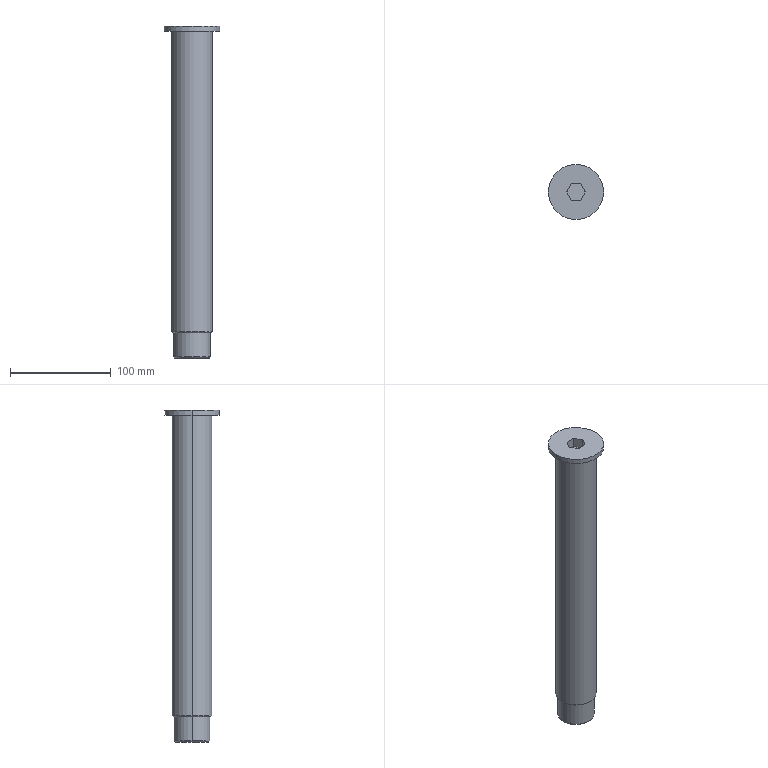Part | SolidWorks | features ICE 4, Chamfer 2, Fillet 2, Extrusion 1 | 1 solid | 32 faces | box 55 x 55 x 330 mm | volume 411254 mm3 | plane 14 | cylinder 11 | cone 5 | torus 2 | commonest cylinder face diameters 1 x4 36 x3 40 x2 55 x2
STEP:
#1=CARTESIAN_POINT('',(-20.5,0.,325.));
#2=VERTEX_POINT('',#1);
#3=CARTESIAN_POINT('',(20.5,0.,325.));
#4=VERTEX_POINT('',#3);
#5=CARTESIAN_POINT('',(0.,0.,325.));
#6=DIRECTION('',(0.,0.,1.));
#7=DIRECTION('',(1.,0.,0.));
#8=AXIS2_PLACEMENT_3D('',#5,#6,#7);
#9=CIRCLE('',#8,20.5);
#10=EDGE_CURVE('',#2,#4,#9,.T.);
#11=ORIENTED_EDGE('',*,*,#10,.F.);
#12=CARTESIAN_POINT('',(-20.,0.,324.5));
#13=VERTEX_POINT('',#12);
#14=CARTESIAN_POINT('',(-20.5,0.,324.5));
#15=DIRECTION('',(0.,1.,0.));
#16=DIRECTION('',(-1.,0.,0.));
#17=AXIS2_PLACEMENT_3D('',#14,#15,#16);
#18=CIRCLE('',#17,0.5);
#19=EDGE_CURVE('',#2,#13,#18,.T.);
#20=ORIENTED_EDGE('',*,*,#19,.T.);
#21=CARTESIAN_POINT('',(20.,0.,324.5));
#22=VERTEX_POINT('',#21);
#23=CARTESIAN_POINT('',(0.,0.,324.5));
#24=DIRECTION('',(0.,0.,-1.));
#25=DIRECTION('',(1.,0.,0.));
#26=AXIS2_PLACEMENT_3D('',#23,#24,#25);
#27=CIRCLE('',#26,20.);
#28=EDGE_CURVE('',#22,#13,#27,.T.);
#29=ORIENTED_EDGE('',*,*,#28,.F.);
#30=CARTESIAN_POINT('',(20.5,0.,324.5));
#31=DIRECTION('',(0.,-1.,0.));
#32=DIRECTION('',(0.,0.,-1.));
#33=AXIS2_PLACEMENT_3D('',#30,#31,#32);
#34=CIRCLE('',#33,0.5);
#35=EDGE_CURVE('',#4,#22,#34,.T.);
#36=ORIENTED_EDGE('',*,*,#35,.F.);
#37=EDGE_LOOP('',(#11,#20,#29,#36));
#38=FACE_OUTER_BOUND('',#37,.T.);
#39=CARTESIAN_POINT('',(0.,0.,324.5));
#40=DIRECTION('',(0.,0.,1.));
#41=DIRECTION('',(1.,0.,0.));
#42=AXIS2_PLACEMENT_3D('',#39,#40,#41);
#43=TOROIDAL_SURFACE('',#42,20.5,0.5);
#44=ADVANCED_FACE('',(#38),#43,.F.);
#45=CARTESIAN_POINT('',(-17.,0.,0.));
#46=VERTEX_POINT('',#45);
#47=CARTESIAN_POINT('',(-3.,16.733,0.));
#48=VERTEX_POINT('',#47);
#49=CARTESIAN_POINT('',(0.,0.,0.));
#50=DIRECTION('',(0.,0.,-1.));
#51=DIRECTION('',(1.,0.,0.));
#52=AXIS2_PLACEMENT_3D('',#49,#50,#51);
#53=CIRCLE('',#52,17.);
#54=EDGE_CURVE('',#46,#48,#53,.T.);
#55=ORIENTED_EDGE('',*,*,#54,.F.);
#56=CARTESIAN_POINT('',(-18.,0.,1.));
#57=VERTEX_POINT('',#56);
#58=CARTESIAN_POINT('',(-17.,0.,0.));
#59=DIRECTION('',(-0.7071,0.,0.7071));
#60=VECTOR('',#59,1000.);
#61=LINE('',#58,#60);
#62=EDGE_CURVE('',#46,#57,#61,.T.);
#63=ORIENTED_EDGE('',*,*,#62,.T.);
#64=CARTESIAN_POINT('',(-3.6,17.636,1.));
#65=VERTEX_POINT('',#64);
#66=CARTESIAN_POINT('',(0.,0.,1.));
#67=DIRECTION('',(0.,0.,1.));
#68=DIRECTION('',(1.,0.,0.));
#69=AXIS2_PLACEMENT_3D('',#66,#67,#68);
#70=CIRCLE('',#69,18.);
#71=EDGE_CURVE('',#65,#57,#70,.T.);
#72=ORIENTED_EDGE('',*,*,#71,.F.);
#73=CARTESIAN_POINT('',(-3.,17.146,0.4069));
#74=VERTEX_POINT('',#73);
#75=CARTESIAN_POINT('',(-3.6,17.636,1.));
#76=CARTESIAN_POINT('',(-3.509,17.655,1.));
#77=CARTESIAN_POINT('',(-3.418,17.647,0.9743));
#78=CARTESIAN_POINT('',(-3.262,17.594,0.8932));
#79=CARTESIAN_POINT('',(-3.198,17.551,0.8399));
#80=CARTESIAN_POINT('',(-3.098,17.452,0.7251));
#81=CARTESIAN_POINT('',(-3.061,17.395,0.6623));
#82=CARTESIAN_POINT('',(-3.013,17.275,0.5357));
#83=CARTESIAN_POINT('',(-3.,17.212,0.4712));
#84=CARTESIAN_POINT('',(-3.,17.146,0.4069));
#85=B_SPLINE_CURVE_WITH_KNOTS('',3,(#75,#76,#77,#78,#79,#80,#81,#82,#83,#84),.UNSPECIFIED.,.F.,.F.,(4,2,2,2,4),(0.,0.0002726,0.0005452,0.0008178,0.00109),.UNSPECIFIED.);
#86=EDGE_CURVE('',#65,#74,#85,.T.);
#87=ORIENTED_EDGE('',*,*,#86,.T.);
#88=CARTESIAN_POINT('',(-3.,16.733,0.));
#89=CARTESIAN_POINT('',(-3.,16.871,0.1356));
#90=CARTESIAN_POINT('',(-3.,17.009,0.2712));
#91=CARTESIAN_POINT('',(-3.,17.146,0.4069));
#92=B_SPLINE_CURVE_WITH_KNOTS('',3,(#88,#89,#90,#91),.UNSPECIFIED.,.F.,.F.,(4,4),(0.007295,0.007875),.UNSPECIFIED.);
#93=EDGE_CURVE('',#48,#74,#92,.T.);
#94=ORIENTED_EDGE('',*,*,#93,.F.);
#95=EDGE_LOOP('',(#55,#63,#72,#87,#94));
#96=FACE_OUTER_BOUND('',#95,.T.);
#97=CARTESIAN_POINT('',(0.,0.,0.));
#98=DIRECTION('',(0.,0.,1.));
#99=DIRECTION('',(1.,0.,0.));
#100=AXIS2_PLACEMENT_3D('',#97,#98,#99);
#101=CONICAL_SURFACE('',#100,17.,0.7854);
#102=ADVANCED_FACE('',(#96),#101,.T.);
#103=ORIENTED_EDGE('',*,*,#62,.F.);
#104=CARTESIAN_POINT('',(17.,0.,0.));
#105=VERTEX_POINT('',#104);
#106=CARTESIAN_POINT('',(0.,0.,0.));
#107=DIRECTION('',(0.,0.,-1.));
#108=DIRECTION('',(1.,0.,0.));
#109=AXIS2_PLACEMENT_3D('',#106,#107,#108);
#110=CIRCLE('',#109,17.);
#111=EDGE_CURVE('',#105,#46,#110,.T.);
#112=ORIENTED_EDGE('',*,*,#111,.F.);
#113=CARTESIAN_POINT('',(18.,0.,1.));
#114=VERTEX_POINT('',#113);
#115=CARTESIAN_POINT('',(17.,0.,0.));
#116=DIRECTION('',(0.7071,0.,0.7071));
#117=VECTOR('',#116,1000.);
#118=LINE('',#115,#117);
#119=EDGE_CURVE('',#105,#114,#118,.T.);
#120=ORIENTED_EDGE('',*,*,#119,.T.);
#121=CARTESIAN_POINT('',(0.,0.,1.));
#122=DIRECTION('',(0.,0.,1.));
#123=DIRECTION('',(1.,0.,0.));
#124=AXIS2_PLACEMENT_3D('',#121,#122,#123);
#125=CIRCLE('',#124,18.);
#126=EDGE_CURVE('',#57,#114,#125,.T.);
#127=ORIENTED_EDGE('',*,*,#126,.F.);
#128=EDGE_LOOP('',(#103,#112,#120,#127));
#129=FACE_OUTER_BOUND('',#128,.T.);
#130=CARTESIAN_POINT('',(0.,0.,0.));
#131=DIRECTION('',(0.,0.,1.));
#132=DIRECTION('',(1.,0.,0.));
#133=AXIS2_PLACEMENT_3D('',#130,#131,#132);
#134=CONICAL_SURFACE('',#133,17.,0.7854);
#135=ADVANCED_FACE('',(#129),#134,.T.);
#136=CARTESIAN_POINT('',(-19.,0.,25.));
#137=VERTEX_POINT('',#136);
#138=CARTESIAN_POINT('',(19.,0.,25.));
#139=VERTEX_POINT('',#138);
#140=CARTESIAN_POINT('',(0.,0.,25.));
#141=DIRECTION('',(0.,0.,-1.));
#142=DIRECTION('',(-1.,0.,0.));
#143=AXIS2_PLACEMENT_3D('',#140,#141,#142);
#144=CIRCLE('',#143,19.);
#145=EDGE_CURVE('',#137,#139,#144,.T.);
#146=ORIENTED_EDGE('',*,*,#145,.F.);
#147=CARTESIAN_POINT('',(-20.,0.,26.));
#148=VERTEX_POINT('',#147);
#149=CARTESIAN_POINT('',(-19.,0.,25.));
#150=DIRECTION('',(-0.7071,0.,0.7071));
#151=VECTOR('',#150,1000.);
#152=LINE('',#149,#151);
#153=EDGE_CURVE('',#137,#148,#152,.T.);
#154=ORIENTED_EDGE('',*,*,#153,.T.);
#155=CARTESIAN_POINT('',(20.,0.,26.));
#156=VERTEX_POINT('',#155);
#157=CARTESIAN_POINT('',(0.,0.,26.));
#158=DIRECTION('',(0.,0.,1.));
#159=DIRECTION('',(-1.,0.,0.));
#160=AXIS2_PLACEMENT_3D('',#157,#158,#159);
#161=CIRCLE('',#160,20.);
#162=EDGE_CURVE('',#156,#148,#161,.T.);
#163=ORIENTED_EDGE('',*,*,#162,.F.);
#164=CARTESIAN_POINT('',(19.,0.,25.));
#165=DIRECTION('',(0.7071,0.,0.7071));
#166=VECTOR('',#165,1000.);
#167=LINE('',#164,#166);
#168=EDGE_CURVE('',#139,#156,#167,.T.);
#169=ORIENTED_EDGE('',*,*,#168,.F.);
#170=EDGE_LOOP('',(#146,#154,#163,#169));
#171=FACE_OUTER_BOUND('',#170,.T.);
#172=CARTESIAN_POINT('',(0.,0.,25.));
#173=DIRECTION('',(0.,0.,1.));
#174=DIRECTION('',(1.,0.,0.));
#175=AXIS2_PLACEMENT_3D('',#172,#173,#174);
#176=CONICAL_SURFACE('',#175,19.,0.7854);
#177=ADVANCED_FACE('',(#171),#176,.T.);
#178=CARTESIAN_POINT('',(3.6,17.636,25.));
#179=VERTEX_POINT('',#178);
#180=CARTESIAN_POINT('',(18.,0.,25.));
#181=VERTEX_POINT('',#180);
#182=CARTESIAN_POINT('',(0.,0.,25.));
#183=DIRECTION('',(0.,0.,-1.));
#184=DIRECTION('',(-1.,0.,0.));
#185=AXIS2_PLACEMENT_3D('',#182,#183,#184);
#186=CIRCLE('',#185,18.);
#187=EDGE_CURVE('',#179,#181,#186,.T.);
#188=ORIENTED_EDGE('',*,*,#187,.T.);
#189=CARTESIAN_POINT('',(18.,0.,25.));
#190=DIRECTION('',(0.,0.,-1.));
#191=VECTOR('',#190,1000.);
#192=LINE('',#189,#191);
#193=EDGE_CURVE('',#181,#114,#192,.T.);
#194=ORIENTED_EDGE('',*,*,#193,.T.);
#195=CARTESIAN_POINT('',(3.6,17.636,1.));
#196=VERTEX_POINT('',#195);
#197=CARTESIAN_POINT('',(0.,0.,1.));
#198=DIRECTION('',(0.,0.,1.));
#199=DIRECTION('',(1.,0.,0.));
#200=AXIS2_PLACEMENT_3D('',#197,#198,#199);
#201=CIRCLE('',#200,18.);
#202=EDGE_CURVE('',#114,#196,#201,.T.);
#203=ORIENTED_EDGE('',*,*,#202,.T.);
#204=CARTESIAN_POINT('',(3.6,17.636,25.));
#205=DIRECTION('',(0.,0.,1.));
#206=VECTOR('',#205,1000.);
#207=LINE('',#204,#206);
#208=EDGE_CURVE('',#196,#179,#207,.T.);
#209=ORIENTED_EDGE('',*,*,#208,.T.);
#210=EDGE_LOOP('',(#188,#194,#203,#209));
#211=FACE_OUTER_BOUND('',#210,.T.);
#212=CARTESIAN_POINT('',(0.,0.,25.));
#213=DIRECTION('',(0.,0.,-1.));
#214=DIRECTION('',(-1.,0.,0.));
#215=AXIS2_PLACEMENT_3D('',#212,#213,#214);
#216=CYLINDRICAL_SURFACE('',#215,18.);
#217=ADVANCED_FACE('',(#211),#216,.T.);
#218=ORIENTED_EDGE('',*,*,#193,.F.);
#219=CARTESIAN_POINT('',(-18.,0.,25.));
#220=VERTEX_POINT('',#219);
#221=CARTESIAN_POINT('',(0.,0.,25.));
#222=DIRECTION('',(0.,0.,-1.));
#223=DIRECTION('',(-1.,0.,0.));
#224=AXIS2_PLACEMENT_3D('',#221,#222,#223);
#225=CIRCLE('',#224,18.);
#226=EDGE_CURVE('',#181,#220,#225,.T.);
#227=ORIENTED_EDGE('',*,*,#226,.T.);
#228=CARTESIAN_POINT('',(-18.,0.,25.));
#229=DIRECTION('',(0.,0.,-1.));
#230=VECTOR('',#229,1000.);
#231=LINE('',#228,#230);
#232=EDGE_CURVE('',#220,#57,#231,.T.);
#233=ORIENTED_EDGE('',*,*,#232,.T.);
#234=ORIENTED_EDGE('',*,*,#126,.T.);
#235=EDGE_LOOP('',(#218,#227,#233,#234));
#236=FACE_OUTER_BOUND('',#235,.T.);
#237=CARTESIAN_POINT('',(0.,0.,25.));
#238=DIRECTION('',(0.,0.,-1.));
#239=DIRECTION('',(-1.,0.,0.));
#240=AXIS2_PLACEMENT_3D('',#237,#238,#239);
#241=CYLINDRICAL_SURFACE('',#240,18.);
#242=ADVANCED_FACE('',(#236),#241,.T.);
#243=CARTESIAN_POINT('',(27.5,0.,330.));
#244=VERTEX_POINT('',#243);
#245=CARTESIAN_POINT('',(-27.5,0.,330.));
#246=VERTEX_POINT('',#245);
#247=CARTESIAN_POINT('',(0.,0.,330.));
#248=DIRECTION('',(0.,0.,1.));
#249=DIRECTION('',(1.,0.,0.));
#250=AXIS2_PLACEMENT_3D('',#247,#248,#249);
#251=CIRCLE('',#250,27.5);
#252=EDGE_CURVE('',#244,#246,#251,.T.);
#253=ORIENTED_EDGE('',*,*,#252,.F.);
#254=CARTESIAN_POINT('',(27.5,0.,325.));
#255=VERTEX_POINT('',#254);
#256=CARTESIAN_POINT('',(27.5,0.,330.));
#257=DIRECTION('',(0.,0.,-1.));
#258=VECTOR('',#257,1000.);
#259=LINE('',#256,#258);
#260=EDGE_CURVE('',#244,#255,#259,.T.);
#261=ORIENTED_EDGE('',*,*,#260,.T.);
#262=CARTESIAN_POINT('',(-27.5,0.,325.));
#263=VERTEX_POINT('',#262);
#264=CARTESIAN_POINT('',(0.,0.,325.));
#265=DIRECTION('',(0.,0.,1.));
#266=DIRECTION('',(1.,0.,0.));
#267=AXIS2_PLACEMENT_3D('',#264,#265,#266);
#268=CIRCLE('',#267,27.5);
#269=EDGE_CURVE('',#255,#263,#268,.T.);
#270=ORIENTED_EDGE('',*,*,#269,.T.);
#271=CARTESIAN_POINT('',(-27.5,0.,330.));
#272=DIRECTION('',(0.,0.,-1.));
#273=VECTOR('',#272,1000.);
#274=LINE('',#271,#273);
#275=EDGE_CURVE('',#246,#263,#274,.T.);
#276=ORIENTED_EDGE('',*,*,#275,.F.);
#277=EDGE_LOOP('',(#253,#261,#270,#276));
#278=FACE_OUTER_BOUND('',#277,.T.);
#279=CARTESIAN_POINT('',(0.,0.,330.));
#280=DIRECTION('',(0.,0.,-1.));
#281=DIRECTION('',(-1.,0.,0.));
#282=AXIS2_PLACEMENT_3D('',#279,#280,#281);
#283=CYLINDRICAL_SURFACE('',#282,27.5);
#284=ADVANCED_FACE('',(#278),#283,.T.);
#285=CARTESIAN_POINT('',(0.,0.,324.5));
#286=DIRECTION('',(0.,0.,-1.));
#287=DIRECTION('',(1.,0.,0.));
#288=AXIS2_PLACEMENT_3D('',#285,#286,#287);
#289=CIRCLE('',#288,20.);
#290=EDGE_CURVE('',#13,#22,#289,.T.);
#291=ORIENTED_EDGE('',*,*,#290,.T.);
#292=CARTESIAN_POINT('',(20.,0.,325.));
#293=DIRECTION('',(0.,0.,-1.));
#294=VECTOR('',#293,1000.);
#295=LINE('',#292,#294);
#296=EDGE_CURVE('',#22,#156,#295,.T.);
#297=ORIENTED_EDGE('',*,*,#296,.T.);
#298=ORIENTED_EDGE('',*,*,#162,.T.);
#299=CARTESIAN_POINT('',(-20.,0.,325.));
#300=DIRECTION('',(0.,0.,-1.));
#301=VECTOR('',#300,1000.);
#302=LINE('',#299,#301);
#303=EDGE_CURVE('',#13,#148,#302,.T.);
#304=ORIENTED_EDGE('',*,*,#303,.F.);
#305=EDGE_LOOP('',(#291,#297,#298,#304));
#306=FACE_OUTER_BOUND('',#305,.T.);
#307=CARTESIAN_POINT('',(0.,0.,325.));
#308=DIRECTION('',(0.,0.,-1.));
#309=DIRECTION('',(-1.,0.,0.));
#310=AXIS2_PLACEMENT_3D('',#307,#308,#309);
#311=CYLINDRICAL_SURFACE('',#310,20.);
#312=ADVANCED_FACE('',(#306),#311,.T.);
#313=ORIENTED_EDGE('',*,*,#296,.F.);
#314=ORIENTED_EDGE('',*,*,#28,.T.);
#315=ORIENTED_EDGE('',*,*,#303,.T.);
#316=CARTESIAN_POINT('',(0.,0.,26.));
#317=DIRECTION('',(0.,0.,1.));
#318=DIRECTION('',(-1.,0.,0.));
#319=AXIS2_PLACEMENT_3D('',#316,#317,#318);
#320=CIRCLE('',#319,20.);
#321=EDGE_CURVE('',#148,#156,#320,.T.);
#322=ORIENTED_EDGE('',*,*,#321,.T.);
#323=EDGE_LOOP('',(#313,#314,#315,#322));
#324=FACE_OUTER_BOUND('',#323,.T.);
#325=CARTESIAN_POINT('',(0.,0.,325.));
#326=DIRECTION('',(0.,0.,-1.));
#327=DIRECTION('',(-1.,0.,0.));
#328=AXIS2_PLACEMENT_3D('',#325,#326,#327);
#329=CYLINDRICAL_SURFACE('',#328,20.);
#330=ADVANCED_FACE('',(#324),#329,.T.);
#331=ORIENTED_EDGE('',*,*,#260,.F.);
#332=CARTESIAN_POINT('',(0.,0.,330.));
#333=DIRECTION('',(0.,0.,1.));
#334=DIRECTION('',(1.,0.,0.));
#335=AXIS2_PLACEMENT_3D('',#332,#333,#334);
#336=CIRCLE('',#335,27.5);
#337=EDGE_CURVE('',#246,#244,#336,.T.);
#338=ORIENTED_EDGE('',*,*,#337,.F.);
#339=ORIENTED_EDGE('',*,*,#275,.T.);
#340=CARTESIAN_POINT('',(0.,0.,325.));
#341=DIRECTION('',(0.,0.,1.));
#342=DIRECTION('',(1.,0.,0.));
#343=AXIS2_PLACEMENT_3D('',#340,#341,#342);
#344=CIRCLE('',#343,27.5);
#345=EDGE_CURVE('',#263,#255,#344,.T.);
#346=ORIENTED_EDGE('',*,*,#345,.T.);
#347=EDGE_LOOP('',(#331,#338,#339,#346));
#348=FACE_OUTER_BOUND('',#347,.T.);
#349=CARTESIAN_POINT('',(0.,0.,330.));
#350=DIRECTION('',(0.,0.,-1.));
#351=DIRECTION('',(-1.,0.,0.));
#352=AXIS2_PLACEMENT_3D('',#349,#350,#351);
#353=CYLINDRICAL_SURFACE('',#352,27.5);
#354=ADVANCED_FACE('',(#348),#353,.T.);
#355=CARTESIAN_POINT('',(4.619,-8.,330.));
#356=VERTEX_POINT('',#355);
#357=CARTESIAN_POINT('',(9.238,0.,330.));
#358=VERTEX_POINT('',#357);
#359=CARTESIAN_POINT('',(4.619,-8.,330.));
#360=DIRECTION('',(0.5,0.866,0.));
#361=VECTOR('',#360,1000.);
#362=LINE('',#359,#361);
#363=EDGE_CURVE('',#356,#358,#362,.T.);
#364=ORIENTED_EDGE('',*,*,#363,.F.);
#365=CARTESIAN_POINT('',(-4.619,-8.,330.));
#366=VERTEX_POINT('',#365);
#367=CARTESIAN_POINT('',(-4.619,-8.,330.));
#368=DIRECTION('',(1.,0.,0.));
#369=VECTOR('',#368,1000.);
#370=LINE('',#367,#369);
#371=EDGE_CURVE('',#366,#356,#370,.T.);
#372=ORIENTED_EDGE('',*,*,#371,.F.);
#373=CARTESIAN_POINT('',(-9.238,0.,330.));
#374=VERTEX_POINT('',#373);
#375=CARTESIAN_POINT('',(-9.238,0.,330.));
#376=DIRECTION('',(0.5,-0.866,0.));
#377=VECTOR('',#376,1000.);
#378=LINE('',#375,#377);
#379=EDGE_CURVE('',#374,#366,#378,.T.);
#380=ORIENTED_EDGE('',*,*,#379,.F.);
#381=CARTESIAN_POINT('',(-4.619,8.,330.));
#382=VERTEX_POINT('',#381);
#383=CARTESIAN_POINT('',(-4.619,8.,330.));
#384=DIRECTION('',(-0.5,-0.866,0.));
#385=VECTOR('',#384,1000.);
#386=LINE('',#383,#385);
#387=EDGE_CURVE('',#382,#374,#386,.T.);
#388=ORIENTED_EDGE('',*,*,#387,.F.);
#389=CARTESIAN_POINT('',(4.619,8.,330.));
#390=VERTEX_POINT('',#389);
#391=CARTESIAN_POINT('',(4.619,8.,330.));
#392=DIRECTION('',(-1.,0.,0.));
#393=VECTOR('',#392,1000.);
#394=LINE('',#391,#393);
#395=EDGE_CURVE('',#390,#382,#394,.T.);
#396=ORIENTED_EDGE('',*,*,#395,.F.);
#397=CARTESIAN_POINT('',(9.238,0.,330.));
#398=DIRECTION('',(-0.5,0.866,0.));
#399=VECTOR('',#398,1000.);
#400=LINE('',#397,#399);
#401=EDGE_CURVE('',#358,#390,#400,.T.);
#402=ORIENTED_EDGE('',*,*,#401,.F.);
#403=EDGE_LOOP('',(#364,#372,#380,#388,#396,#402));
#404=FACE_BOUND('',#403,.T.);
#405=ORIENTED_EDGE('',*,*,#337,.T.);
#406=ORIENTED_EDGE('',*,*,#252,.T.);
#407=EDGE_LOOP('',(#405,#406));
#408=FACE_OUTER_BOUND('',#407,.T.);
#409=CARTESIAN_POINT('',(0.,0.,330.));
#410=DIRECTION('',(0.,0.,1.));
#411=DIRECTION('',(1.,0.,0.));
#412=AXIS2_PLACEMENT_3D('',#409,#410,#411);
#413=PLANE('',#412);
#414=ADVANCED_FACE('',(#404,#408),#413,.T.);
#415=CARTESIAN_POINT('',(0.,0.,325.));
#416=DIRECTION('',(0.,0.,1.));
#417=DIRECTION('',(1.,0.,0.));
#418=AXIS2_PLACEMENT_3D('',#415,#416,#417);
#419=CIRCLE('',#418,20.5);
#420=EDGE_CURVE('',#4,#2,#419,.T.);
#421=ORIENTED_EDGE('',*,*,#420,.T.);
#422=ORIENTED_EDGE('',*,*,#10,.T.);
#423=EDGE_LOOP('',(#421,#422));
#424=FACE_BOUND('',#423,.T.);
#425=ORIENTED_EDGE('',*,*,#345,.F.);
#426=ORIENTED_EDGE('',*,*,#269,.F.);
#427=EDGE_LOOP('',(#425,#426));
#428=FACE_OUTER_BOUND('',#427,.T.);
#429=CARTESIAN_POINT('',(0.,0.,325.));
#430=DIRECTION('',(0.,0.,1.));
#431=DIRECTION('',(1.,0.,0.));
#432=AXIS2_PLACEMENT_3D('',#429,#430,#431);
#433=PLANE('',#432);
#434=ADVANCED_FACE('',(#424,#428),#433,.F.);
#435=ORIENTED_EDGE('',*,*,#363,.T.);
#436=CARTESIAN_POINT('',(9.238,0.,320.));
#437=VERTEX_POINT('',#436);
#438=CARTESIAN_POINT('',(9.238,0.,320.));
#439=DIRECTION('',(0.,0.,1.));
#440=VECTOR('',#439,1000.);
#441=LINE('',#438,#440);
#442=EDGE_CURVE('',#437,#358,#441,.T.);
#443=ORIENTED_EDGE('',*,*,#442,.F.);
#444=CARTESIAN_POINT('',(4.619,-8.,320.));
#445=VERTEX_POINT('',#444);
#446=CARTESIAN_POINT('',(4.619,-8.,320.));
#447=DIRECTION('',(0.5,0.866,0.));
#448=VECTOR('',#447,1000.);
#449=LINE('',#446,#448);
#450=EDGE_CURVE('',#445,#437,#449,.T.);
#451=ORIENTED_EDGE('',*,*,#450,.F.);
#452=CARTESIAN_POINT('',(4.619,-8.,320.));
#453=DIRECTION('',(0.,0.,1.));
#454=VECTOR('',#453,1000.);
#455=LINE('',#452,#454);
#456=EDGE_CURVE('',#445,#356,#455,.T.);
#457=ORIENTED_EDGE('',*,*,#456,.T.);
#458=EDGE_LOOP('',(#435,#443,#451,#457));
#459=FACE_OUTER_BOUND('',#458,.T.);
#460=CARTESIAN_POINT('',(4.619,-8.,320.));
#461=DIRECTION('',(0.866,-0.5,0.));
#462=DIRECTION('',(0.5,0.866,0.));
#463=AXIS2_PLACEMENT_3D('',#460,#461,#462);
#464=PLANE('',#463);
#465=ADVANCED_FACE('',(#459),#464,.F.);
#466=ORIENTED_EDGE('',*,*,#371,.T.);
#467=ORIENTED_EDGE('',*,*,#456,.F.);
#468=CARTESIAN_POINT('',(-4.619,-8.,320.));
#469=VERTEX_POINT('',#468);
#470=CARTESIAN_POINT('',(-4.619,-8.,320.));
#471=DIRECTION('',(1.,0.,0.));
#472=VECTOR('',#471,1000.);
#473=LINE('',#470,#472);
#474=EDGE_CURVE('',#469,#445,#473,.T.);
#475=ORIENTED_EDGE('',*,*,#474,.F.);
#476=CARTESIAN_POINT('',(-4.619,-8.,320.));
#477=DIRECTION('',(0.,0.,1.));
#478=VECTOR('',#477,1000.);
#479=LINE('',#476,#478);
#480=EDGE_CURVE('',#469,#366,#479,.T.);
#481=ORIENTED_EDGE('',*,*,#480,.T.);
#482=EDGE_LOOP('',(#466,#467,#475,#481));
#483=FACE_OUTER_BOUND('',#482,.T.);
#484=CARTESIAN_POINT('',(-4.619,-8.,320.));
#485=DIRECTION('',(0.,-1.,0.));
#486=DIRECTION('',(1.,0.,0.));
#487=AXIS2_PLACEMENT_3D('',#484,#485,#486);
#488=PLANE('',#487);
#489=ADVANCED_FACE('',(#483),#488,.F.);
#490=ORIENTED_EDGE('',*,*,#379,.T.);
#491=ORIENTED_EDGE('',*,*,#480,.F.);
#492=CARTESIAN_POINT('',(-9.238,0.,320.));
#493=VERTEX_POINT('',#492);
#494=CARTESIAN_POINT('',(-9.238,0.,320.));
#495=DIRECTION('',(0.5,-0.866,0.));
#496=VECTOR('',#495,1000.);
#497=LINE('',#494,#496);
#498=EDGE_CURVE('',#493,#469,#497,.T.);
#499=ORIENTED_EDGE('',*,*,#498,.F.);
#500=CARTESIAN_POINT('',(-9.238,0.,320.));
#501=DIRECTION('',(0.,0.,1.));
#502=VECTOR('',#501,1000.);
#503=LINE('',#500,#502);
#504=EDGE_CURVE('',#493,#374,#503,.T.);
#505=ORIENTED_EDGE('',*,*,#504,.T.);
#506=EDGE_LOOP('',(#490,#491,#499,#505));
#507=FACE_OUTER_BOUND('',#506,.T.);
#508=CARTESIAN_POINT('',(-9.238,0.,320.));
#509=DIRECTION('',(-0.866,-0.5,0.));
#510=DIRECTION('',(0.5,-0.866,0.));
#511=AXIS2_PLACEMENT_3D('',#508,#509,#510);
#512=PLANE('',#511);
#513=ADVANCED_FACE('',(#507),#512,.F.);
#514=ORIENTED_EDGE('',*,*,#387,.T.);
#515=ORIENTED_EDGE('',*,*,#504,.F.);
#516=CARTESIAN_POINT('',(-4.619,8.,320.));
#517=VERTEX_POINT('',#516);
#518=CARTESIAN_POINT('',(-4.619,8.,320.));
#519=DIRECTION('',(-0.5,-0.866,0.));
#520=VECTOR('',#519,1000.);
#521=LINE('',#518,#520);
#522=EDGE_CURVE('',#517,#493,#521,.T.);
#523=ORIENTED_EDGE('',*,*,#522,.F.);
#524=CARTESIAN_POINT('',(-4.619,8.,320.));
#525=DIRECTION('',(0.,0.,1.));
#526=VECTOR('',#525,1000.);
#527=LINE('',#524,#526);
#528=EDGE_CURVE('',#517,#382,#527,.T.);
#529=ORIENTED_EDGE('',*,*,#528,.T.);
#530=EDGE_LOOP('',(#514,#515,#523,#529));
#531=FACE_OUTER_BOUND('',#530,.T.);
#532=CARTESIAN_POINT('',(-4.619,8.,320.));
#533=DIRECTION('',(-0.866,0.5,0.));
#534=DIRECTION('',(-0.5,-0.866,0.));
#535=AXIS2_PLACEMENT_3D('',#532,#533,#534);
#536=PLANE('',#535);
#537=ADVANCED_FACE('',(#531),#536,.F.);
#538=ORIENTED_EDGE('',*,*,#395,.T.);
#539=ORIENTED_EDGE('',*,*,#528,.F.);
#540=CARTESIAN_POINT('',(4.619,8.,320.));
#541=VERTEX_POINT('',#540);
#542=CARTESIAN_POINT('',(4.619,8.,320.));
#543=DIRECTION('',(-1.,0.,0.));
#544=VECTOR('',#543,1000.);
#545=LINE('',#542,#544);
#546=EDGE_CURVE('',#541,#517,#545,.T.);
#547=ORIENTED_EDGE('',*,*,#546,.F.);
#548=CARTESIAN_POINT('',(4.619,8.,320.));
#549=DIRECTION('',(0.,0.,1.));
#550=VECTOR('',#549,1000.);
#551=LINE('',#548,#550);
#552=EDGE_CURVE('',#541,#390,#551,.T.);
#553=ORIENTED_EDGE('',*,*,#552,.T.);
#554=EDGE_LOOP('',(#538,#539,#547,#553));
#555=FACE_OUTER_BOUND('',#554,.T.);
#556=CARTESIAN_POINT('',(4.619,8.,320.));
#557=DIRECTION('',(0.,1.,0.));
#558=DIRECTION('',(0.,0.,1.));
#559=AXIS2_PLACEMENT_3D('',#556,#557,#558);
#560=PLANE('',#559);
#561=ADVANCED_FACE('',(#555),#560,.F.);
#562=ORIENTED_EDGE('',*,*,#401,.T.);
#563=ORIENTED_EDGE('',*,*,#552,.F.);
#564=CARTESIAN_POINT('',(9.238,0.,320.));
#565=DIRECTION('',(-0.5,0.866,0.));
#566=VECTOR('',#565,1000.);
#567=LINE('',#564,#566);
#568=EDGE_CURVE('',#437,#541,#567,.T.);
#569=ORIENTED_EDGE('',*,*,#568,.F.);
#570=ORIENTED_EDGE('',*,*,#442,.T.);
#571=EDGE_LOOP('',(#562,#563,#569,#570));
#572=FACE_OUTER_BOUND('',#571,.T.);
#573=CARTESIAN_POINT('',(9.238,0.,320.));
#574=DIRECTION('',(0.866,0.5,0.));
#575=DIRECTION('',(-0.5,0.866,0.));
#576=AXIS2_PLACEMENT_3D('',#573,#574,#575);
#577=PLANE('',#576);
#578=ADVANCED_FACE('',(#572),#577,.F.);
#579=ORIENTED_EDGE('',*,*,#450,.T.);
#580=ORIENTED_EDGE('',*,*,#568,.T.);
#581=ORIENTED_EDGE('',*,*,#546,.T.);
#582=ORIENTED_EDGE('',*,*,#522,.T.);
#583=ORIENTED_EDGE('',*,*,#498,.T.);
#584=ORIENTED_EDGE('',*,*,#474,.T.);
#585=EDGE_LOOP('',(#579,#580,#581,#582,#583,#584));
#586=FACE_OUTER_BOUND('',#585,.T.);
#587=CARTESIAN_POINT('',(0.,0.,320.));
#588=DIRECTION('',(0.,0.,1.));
#589=DIRECTION('',(1.,0.,0.));
#590=AXIS2_PLACEMENT_3D('',#587,#588,#589);
#591=PLANE('',#590);
#592=ADVANCED_FACE('',(#586),#591,.T.);
#593=CARTESIAN_POINT('',(0.,0.,25.));
#594=DIRECTION('',(0.,0.,-1.));
#595=DIRECTION('',(-1.,0.,0.));
#596=AXIS2_PLACEMENT_3D('',#593,#594,#595);
#597=CIRCLE('',#596,19.);
#598=EDGE_CURVE('',#139,#137,#597,.T.);
#599=ORIENTED_EDGE('',*,*,#598,.T.);
#600=ORIENTED_EDGE('',*,*,#145,.T.);
#601=EDGE_LOOP('',(#599,#600));
#602=FACE_OUTER_BOUND('',#601,.T.);
#603=CARTESIAN_POINT('',(-2.5,13.,25.));
#604=VERTEX_POINT('',#603);
#605=CARTESIAN_POINT('',(2.5,13.,25.));
#606=VERTEX_POINT('',#605);
#607=CARTESIAN_POINT('',(3.,13.,25.));
#608=DIRECTION('',(1.,0.,0.));
#609=VECTOR('',#608,1000.);
#610=LINE('',#607,#609);
#611=EDGE_CURVE('',#604,#606,#610,.T.);
#612=ORIENTED_EDGE('',*,*,#611,.F.);
#613=CARTESIAN_POINT('',(-3.,13.5,25.));
#614=VERTEX_POINT('',#613);
#615=CARTESIAN_POINT('',(-2.5,13.5,25.));
#616=DIRECTION('',(0.,0.,-1.));
#617=DIRECTION('',(-1.,0.,0.));
#618=AXIS2_PLACEMENT_3D('',#615,#616,#617);
#619=CIRCLE('',#618,0.5);
#620=EDGE_CURVE('',#604,#614,#619,.T.);
#621=ORIENTED_EDGE('',*,*,#620,.T.);
#622=CARTESIAN_POINT('',(-3.,17.146,25.));
#623=VERTEX_POINT('',#622);
#624=CARTESIAN_POINT('',(-3.,23.,25.));
#625=DIRECTION('',(0.,-1.,0.));
#626=VECTOR('',#625,1000.);
#627=LINE('',#624,#626);
#628=EDGE_CURVE('',#623,#614,#627,.T.);
#629=ORIENTED_EDGE('',*,*,#628,.F.);
#630=CARTESIAN_POINT('',(-3.6,17.636,25.));
#631=VERTEX_POINT('',#630);
#632=CARTESIAN_POINT('',(-3.5,17.146,25.));
#633=DIRECTION('',(0.,0.,1.));
#634=DIRECTION('',(-1.,0.,0.));
#635=AXIS2_PLACEMENT_3D('',#632,#633,#634);
#636=CIRCLE('',#635,0.5);
#637=EDGE_CURVE('',#623,#631,#636,.T.);
#638=ORIENTED_EDGE('',*,*,#637,.T.);
#639=CARTESIAN_POINT('',(0.,0.,25.));
#640=DIRECTION('',(0.,0.,-1.));
#641=DIRECTION('',(-1.,0.,0.));
#642=AXIS2_PLACEMENT_3D('',#639,#640,#641);
#643=CIRCLE('',#642,18.);
#644=EDGE_CURVE('',#220,#631,#643,.T.);
#645=ORIENTED_EDGE('',*,*,#644,.F.);
#646=ORIENTED_EDGE('',*,*,#226,.F.);
#647=ORIENTED_EDGE('',*,*,#187,.F.);
#648=CARTESIAN_POINT('',(3.,17.146,25.));
#649=VERTEX_POINT('',#648);
#650=CARTESIAN_POINT('',(3.5,17.146,25.));
#651=DIRECTION('',(0.,0.,1.));
#652=DIRECTION('',(-1.,0.,0.));
#653=AXIS2_PLACEMENT_3D('',#650,#651,#652);
#654=CIRCLE('',#653,0.5);
#655=EDGE_CURVE('',#179,#649,#654,.T.);
#656=ORIENTED_EDGE('',*,*,#655,.T.);
#657=CARTESIAN_POINT('',(3.,13.5,25.));
#658=VERTEX_POINT('',#657);
#659=CARTESIAN_POINT('',(3.,23.,25.));
#660=DIRECTION('',(0.,1.,0.));
#661=VECTOR('',#660,1000.);
#662=LINE('',#659,#661);
#663=EDGE_CURVE('',#658,#649,#662,.T.);
#664=ORIENTED_EDGE('',*,*,#663,.F.);
#665=CARTESIAN_POINT('',(2.5,13.5,25.));
#666=DIRECTION('',(0.,0.,-1.));
#667=DIRECTION('',(-1.,0.,0.));
#668=AXIS2_PLACEMENT_3D('',#665,#666,#667);
#669=CIRCLE('',#668,0.5);
#670=EDGE_CURVE('',#658,#606,#669,.T.);
#671=ORIENTED_EDGE('',*,*,#670,.T.);
#672=EDGE_LOOP('',(#612,#621,#629,#638,#645,#646,#647,#656,#664,#671));
#673=FACE_BOUND('',#672,.T.);
#674=CARTESIAN_POINT('',(0.,0.,25.));
#675=DIRECTION('',(0.,0.,-1.));
#676=DIRECTION('',(-1.,0.,0.));
#677=AXIS2_PLACEMENT_3D('',#674,#675,#676);
#678=PLANE('',#677);
#679=ADVANCED_FACE('',(#602,#673),#678,.T.);
#680=ORIENTED_EDGE('',*,*,#232,.F.);
#681=ORIENTED_EDGE('',*,*,#644,.T.);
#682=CARTESIAN_POINT('',(-3.6,17.636,25.));
#683=DIRECTION('',(0.,0.,-1.));
#684=VECTOR('',#683,1000.);
#685=LINE('',#682,#684);
#686=EDGE_CURVE('',#631,#65,#685,.T.);
#687=ORIENTED_EDGE('',*,*,#686,.T.);
#688=ORIENTED_EDGE('',*,*,#71,.T.);
#689=EDGE_LOOP('',(#680,#681,#687,#688));
#690=FACE_OUTER_BOUND('',#689,.T.);
#691=CARTESIAN_POINT('',(0.,0.,25.));
#692=DIRECTION('',(0.,0.,-1.));
#693=DIRECTION('',(-1.,0.,0.));
#694=AXIS2_PLACEMENT_3D('',#691,#692,#693);
#695=CYLINDRICAL_SURFACE('',#694,18.);
#696=ADVANCED_FACE('',(#690),#695,.T.);
#697=CARTESIAN_POINT('',(3.,16.733,0.));
#698=VERTEX_POINT('',#697);
#699=CARTESIAN_POINT('',(0.,0.,0.));
#700=DIRECTION('',(0.,0.,-1.));
#701=DIRECTION('',(1.,0.,0.));
#702=AXIS2_PLACEMENT_3D('',#699,#700,#701);
#703=CIRCLE('',#702,17.);
#704=EDGE_CURVE('',#698,#105,#703,.T.);
#705=ORIENTED_EDGE('',*,*,#704,.T.);
#706=ORIENTED_EDGE('',*,*,#111,.T.);
#707=ORIENTED_EDGE('',*,*,#54,.T.);
#708=CARTESIAN_POINT('',(-3.,13.5,0.));
#709=VERTEX_POINT('',#708);
#710=CARTESIAN_POINT('',(-3.,23.,0.));
#711=DIRECTION('',(0.,1.,0.));
#712=VECTOR('',#711,1000.);
#713=LINE('',#710,#712);
#714=EDGE_CURVE('',#709,#48,#713,.T.);
#715=ORIENTED_EDGE('',*,*,#714,.F.);
#716=CARTESIAN_POINT('',(-2.5,13.,0.));
#717=VERTEX_POINT('',#716);
#718=CARTESIAN_POINT('',(-2.5,13.5,0.));
#719=DIRECTION('',(0.,0.,1.));
#720=DIRECTION('',(1.,0.,0.));
#721=AXIS2_PLACEMENT_3D('',#718,#719,#720);
#722=CIRCLE('',#721,0.5);
#723=EDGE_CURVE('',#709,#717,#722,.T.);
#724=ORIENTED_EDGE('',*,*,#723,.T.);
#725=CARTESIAN_POINT('',(2.5,13.,0.));
#726=VERTEX_POINT('',#725);
#727=CARTESIAN_POINT('',(3.,13.,0.));
#728=DIRECTION('',(-1.,0.,0.));
#729=VECTOR('',#728,1000.);
#730=LINE('',#727,#729);
#731=EDGE_CURVE('',#726,#717,#730,.T.);
#732=ORIENTED_EDGE('',*,*,#731,.F.);
#733=CARTESIAN_POINT('',(3.,13.5,0.));
#734=VERTEX_POINT('',#733);
#735=CARTESIAN_POINT('',(2.5,13.5,0.));
#736=DIRECTION('',(0.,0.,1.));
#737=DIRECTION('',(1.,0.,0.));
#738=AXIS2_PLACEMENT_3D('',#735,#736,#737);
#739=CIRCLE('',#738,0.5);
#740=EDGE_CURVE('',#726,#734,#739,.T.);
#741=ORIENTED_EDGE('',*,*,#740,.T.);
#742=CARTESIAN_POINT('',(3.,23.,0.));
#743=DIRECTION('',(0.,-1.,0.));
#744=VECTOR('',#743,1000.);
#745=LINE('',#742,#744);
#746=EDGE_CURVE('',#698,#734,#745,.T.);
#747=ORIENTED_EDGE('',*,*,#746,.F.);
#748=EDGE_LOOP('',(#705,#706,#707,#715,#724,#732,#741,#747));
#749=FACE_OUTER_BOUND('',#748,.T.);
#750=CARTESIAN_POINT('',(0.,0.,0.));
#751=DIRECTION('',(0.,0.,1.));
#752=DIRECTION('',(1.,0.,0.));
#753=AXIS2_PLACEMENT_3D('',#750,#751,#752);
#754=PLANE('',#753);
#755=ADVANCED_FACE('',(#749),#754,.F.);
#756=ORIENTED_EDGE('',*,*,#153,.F.);
#757=ORIENTED_EDGE('',*,*,#598,.F.);
#758=ORIENTED_EDGE('',*,*,#168,.T.);
#759=ORIENTED_EDGE('',*,*,#321,.F.);
#760=EDGE_LOOP('',(#756,#757,#758,#759));
#761=FACE_OUTER_BOUND('',#760,.T.);
#762=CARTESIAN_POINT('',(0.,0.,25.));
#763=DIRECTION('',(0.,0.,1.));
#764=DIRECTION('',(1.,0.,0.));
#765=AXIS2_PLACEMENT_3D('',#762,#763,#764);
#766=CONICAL_SURFACE('',#765,19.,0.7854);
#767=ADVANCED_FACE('',(#761),#766,.T.);
#768=ORIENTED_EDGE('',*,*,#119,.F.);
#769=ORIENTED_EDGE('',*,*,#704,.F.);
#770=CARTESIAN_POINT('',(3.,17.146,0.4069));
#771=VERTEX_POINT('',#770);
#772=CARTESIAN_POINT('',(3.,17.146,0.4069));
#773=CARTESIAN_POINT('',(3.,17.009,0.2712));
#774=CARTESIAN_POINT('',(3.,16.871,0.1356));
#775=CARTESIAN_POINT('',(3.,16.733,0.));
#776=B_SPLINE_CURVE_WITH_KNOTS('',3,(#772,#773,#774,#775),.UNSPECIFIED.,.F.,.F.,(4,4),(0.008096,0.008676),.UNSPECIFIED.);
#777=EDGE_CURVE('',#771,#698,#776,.T.);
#778=ORIENTED_EDGE('',*,*,#777,.F.);
#779=CARTESIAN_POINT('',(3.,17.146,0.4069));
#780=CARTESIAN_POINT('',(3.,17.212,0.4712));
#781=CARTESIAN_POINT('',(3.012,17.274,0.5351));
#782=CARTESIAN_POINT('',(3.061,17.395,0.6621));
#783=CARTESIAN_POINT('',(3.098,17.452,0.7245));
#784=CARTESIAN_POINT('',(3.198,17.551,0.8398));
#785=CARTESIAN_POINT('',(3.262,17.594,0.8934));
#786=CARTESIAN_POINT('',(3.417,17.646,0.9741));
#787=CARTESIAN_POINT('',(3.509,17.655,1.));
#788=CARTESIAN_POINT('',(3.6,17.636,1.));
#789=B_SPLINE_CURVE_WITH_KNOTS('',3,(#779,#780,#781,#782,#783,#784,#785,#786,#787,#788),.UNSPECIFIED.,.F.,.F.,(4,2,2,2,4),(0.,0.000271,0.0005419,0.0008129,0.001084),.UNSPECIFIED.);
#790=EDGE_CURVE('',#771,#196,#789,.T.);
#791=ORIENTED_EDGE('',*,*,#790,.T.);
#792=ORIENTED_EDGE('',*,*,#202,.F.);
#793=EDGE_LOOP('',(#768,#769,#778,#791,#792));
#794=FACE_OUTER_BOUND('',#793,.T.);
#795=CARTESIAN_POINT('',(0.,0.,0.));
#796=DIRECTION('',(0.,0.,1.));
#797=DIRECTION('',(1.,0.,0.));
#798=AXIS2_PLACEMENT_3D('',#795,#796,#797);
#799=CONICAL_SURFACE('',#798,17.,0.7854);
#800=ADVANCED_FACE('',(#794),#799,.T.);
#801=ORIENTED_EDGE('',*,*,#19,.F.);
#802=ORIENTED_EDGE('',*,*,#420,.F.);
#803=ORIENTED_EDGE('',*,*,#35,.T.);
#804=ORIENTED_EDGE('',*,*,#290,.F.);
#805=EDGE_LOOP('',(#801,#802,#803,#804));
#806=FACE_OUTER_BOUND('',#805,.T.);
#807=CARTESIAN_POINT('',(0.,0.,324.5));
#808=DIRECTION('',(0.,0.,1.));
#809=DIRECTION('',(1.,0.,0.));
#810=AXIS2_PLACEMENT_3D('',#807,#808,#809);
#811=TOROIDAL_SURFACE('',#810,20.5,0.5);
#812=ADVANCED_FACE('',(#806),#811,.F.);
#813=ORIENTED_EDGE('',*,*,#628,.T.);
#814=CARTESIAN_POINT('',(-3.,13.5,0.));
#815=DIRECTION('',(0.,0.,-1.));
#816=VECTOR('',#815,1000.);
#817=LINE('',#814,#816);
#818=EDGE_CURVE('',#614,#709,#817,.T.);
#819=ORIENTED_EDGE('',*,*,#818,.T.);
#820=ORIENTED_EDGE('',*,*,#714,.T.);
#821=ORIENTED_EDGE('',*,*,#93,.T.);
#822=CARTESIAN_POINT('',(-3.,17.146,25.));
#823=DIRECTION('',(0.,0.,1.));
#824=VECTOR('',#823,1000.);
#825=LINE('',#822,#824);
#826=EDGE_CURVE('',#74,#623,#825,.T.);
#827=ORIENTED_EDGE('',*,*,#826,.T.);
#828=EDGE_LOOP('',(#813,#819,#820,#821,#827));
#829=FACE_OUTER_BOUND('',#828,.T.);
#830=CARTESIAN_POINT('',(-3.,23.,36.662));
#831=DIRECTION('',(-1.,0.,0.));
#832=DIRECTION('',(0.,-1.,0.));
#833=AXIS2_PLACEMENT_3D('',#830,#831,#832);
#834=PLANE('',#833);
#835=ADVANCED_FACE('',(#829),#834,.F.);
#836=ORIENTED_EDGE('',*,*,#731,.T.);
#837=CARTESIAN_POINT('',(-2.5,13.,25.));
#838=DIRECTION('',(0.,0.,1.));
#839=VECTOR('',#838,1000.);
#840=LINE('',#837,#839);
#841=EDGE_CURVE('',#717,#604,#840,.T.);
#842=ORIENTED_EDGE('',*,*,#841,.T.);
#843=ORIENTED_EDGE('',*,*,#611,.T.);
#844=CARTESIAN_POINT('',(2.5,13.,0.));
#845=DIRECTION('',(0.,0.,-1.));
#846=VECTOR('',#845,1000.);
#847=LINE('',#844,#846);
#848=EDGE_CURVE('',#606,#726,#847,.T.);
#849=ORIENTED_EDGE('',*,*,#848,.T.);
#850=EDGE_LOOP('',(#836,#842,#843,#849));
#851=FACE_OUTER_BOUND('',#850,.T.);
#852=CARTESIAN_POINT('',(3.,13.,36.662));
#853=DIRECTION('',(0.,-1.,0.));
#854=DIRECTION('',(0.,0.,-1.));
#855=AXIS2_PLACEMENT_3D('',#852,#853,#854);
#856=PLANE('',#855);
#857=ADVANCED_FACE('',(#851),#856,.F.);
#858=ORIENTED_EDGE('',*,*,#746,.T.);
#859=CARTESIAN_POINT('',(3.,13.5,25.));
#860=DIRECTION('',(0.,0.,1.));
#861=VECTOR('',#860,1000.);
#862=LINE('',#859,#861);
#863=EDGE_CURVE('',#734,#658,#862,.T.);
#864=ORIENTED_EDGE('',*,*,#863,.T.);
#865=ORIENTED_EDGE('',*,*,#663,.T.);
#866=CARTESIAN_POINT('',(3.,17.146,1.));
#867=DIRECTION('',(0.,0.,-1.));
#868=VECTOR('',#867,1000.);
#869=LINE('',#866,#868);
#870=EDGE_CURVE('',#649,#771,#869,.T.);
#871=ORIENTED_EDGE('',*,*,#870,.T.);
#872=ORIENTED_EDGE('',*,*,#777,.T.);
#873=EDGE_LOOP('',(#858,#864,#865,#871,#872));
#874=FACE_OUTER_BOUND('',#873,.T.);
#875=CARTESIAN_POINT('',(3.,23.,36.662));
#876=DIRECTION('',(1.,0.,0.));
#877=DIRECTION('',(0.,1.,0.));
#878=AXIS2_PLACEMENT_3D('',#875,#876,#877);
#879=PLANE('',#878);
#880=ADVANCED_FACE('',(#874),#879,.F.);
#881=ORIENTED_EDGE('',*,*,#620,.F.);
#882=ORIENTED_EDGE('',*,*,#841,.F.);
#883=ORIENTED_EDGE('',*,*,#723,.F.);
#884=ORIENTED_EDGE('',*,*,#818,.F.);
#885=EDGE_LOOP('',(#881,#882,#883,#884));
#886=FACE_OUTER_BOUND('',#885,.T.);
#887=CARTESIAN_POINT('',(-2.5,13.5,36.662));
#888=DIRECTION('',(0.,0.,1.));
#889=DIRECTION('',(1.,0.,0.));
#890=AXIS2_PLACEMENT_3D('',#887,#888,#889);
#891=CYLINDRICAL_SURFACE('',#890,0.5);
#892=ADVANCED_FACE('',(#886),#891,.F.);
#893=ORIENTED_EDGE('',*,*,#670,.F.);
#894=ORIENTED_EDGE('',*,*,#863,.F.);
#895=ORIENTED_EDGE('',*,*,#740,.F.);
#896=ORIENTED_EDGE('',*,*,#848,.F.);
#897=EDGE_LOOP('',(#893,#894,#895,#896));
#898=FACE_OUTER_BOUND('',#897,.T.);
#899=CARTESIAN_POINT('',(2.5,13.5,36.662));
#900=DIRECTION('',(0.,0.,1.));
#901=DIRECTION('',(1.,0.,0.));
#902=AXIS2_PLACEMENT_3D('',#899,#900,#901);
#903=CYLINDRICAL_SURFACE('',#902,0.5);
#904=ADVANCED_FACE('',(#898),#903,.F.);
#905=ORIENTED_EDGE('',*,*,#655,.F.);
#906=ORIENTED_EDGE('',*,*,#208,.F.);
#907=ORIENTED_EDGE('',*,*,#790,.F.);
#908=ORIENTED_EDGE('',*,*,#870,.F.);
#909=EDGE_LOOP('',(#905,#906,#907,#908));
#910=FACE_OUTER_BOUND('',#909,.T.);
#911=CARTESIAN_POINT('',(3.5,17.146,25.));
#912=DIRECTION('',(0.,0.,-1.));
#913=DIRECTION('',(-1.,0.,0.));
#914=AXIS2_PLACEMENT_3D('',#911,#912,#913);
#915=CYLINDRICAL_SURFACE('',#914,0.5);
#916=ADVANCED_FACE('',(#910),#915,.T.);
#917=ORIENTED_EDGE('',*,*,#86,.F.);
#918=ORIENTED_EDGE('',*,*,#686,.F.);
#919=ORIENTED_EDGE('',*,*,#637,.F.);
#920=ORIENTED_EDGE('',*,*,#826,.F.);
#921=EDGE_LOOP('',(#917,#918,#919,#920));
#922=FACE_OUTER_BOUND('',#921,.T.);
#923=CARTESIAN_POINT('',(-3.5,17.146,25.));
#924=DIRECTION('',(0.,0.,-1.));
#925=DIRECTION('',(-1.,0.,0.));
#926=AXIS2_PLACEMENT_3D('',#923,#924,#925);
#927=CYLINDRICAL_SURFACE('',#926,0.5);
#928=ADVANCED_FACE('',(#922),#927,.T.);
#929=CLOSED_SHELL('',(#44,#102,#135,#177,#217,#242,#284,#312,#330,#354,#414,#434,#465,#489,#513,#537,#561,#578,#592,#679,#696,#755,#767,#800,#812,#835,#857,#880,#892,#904,#916,#928));
#930=MANIFOLD_SOLID_BREP('',#929);
#931=CARTESIAN_POINT('',(0.,0.,0.));
#932=DIRECTION('',(0.,0.,1.));
#933=DIRECTION('',(1.,0.,0.));
#934=AXIS2_PLACEMENT_3D('',#931,#932,#933);
#935=(LENGTH_UNIT()NAMED_UNIT(*)SI_UNIT(.MILLI.,.METRE.));
#936=UNCERTAINTY_MEASURE_WITH_UNIT(LENGTH_MEASURE(0.00001),#935,'','');
#937=(NAMED_UNIT(*)PLANE_ANGLE_UNIT()SI_UNIT($,.RADIAN.));
#938=(NAMED_UNIT(*)SI_UNIT($,.STERADIAN.)SOLID_ANGLE_UNIT());
#939=(GEOMETRIC_REPRESENTATION_CONTEXT(3)GLOBAL_UNCERTAINTY_ASSIGNED_CONTEXT((#936))GLOBAL_UNIT_ASSIGNED_CONTEXT((#935,#937,#938))REPRESENTATION_CONTEXT('',''));
#940=ADVANCED_BREP_SHAPE_REPRESENTATION('',(#930,#934),#939);